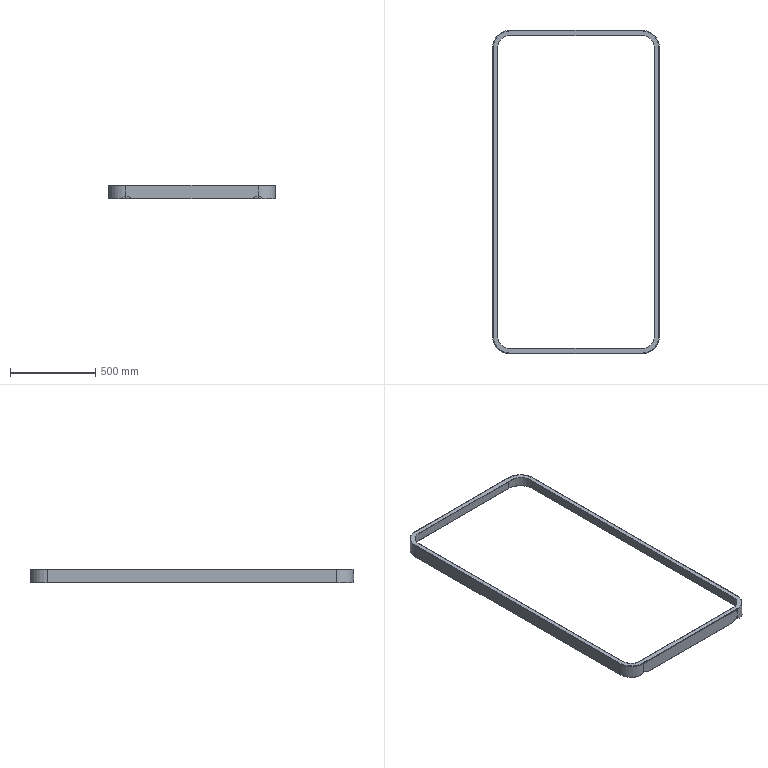Part | STEP file | Split housing part 0301001 | 1 solid | 46 faces | box 980 x 1900 x 80 mm | volume 894741 mm3 | cylinder 22 | plane 16 | torus 8 | commonest cylinder face diameters 3 x4 6 x4 140 x4 197 x4 200 x4 80 x2